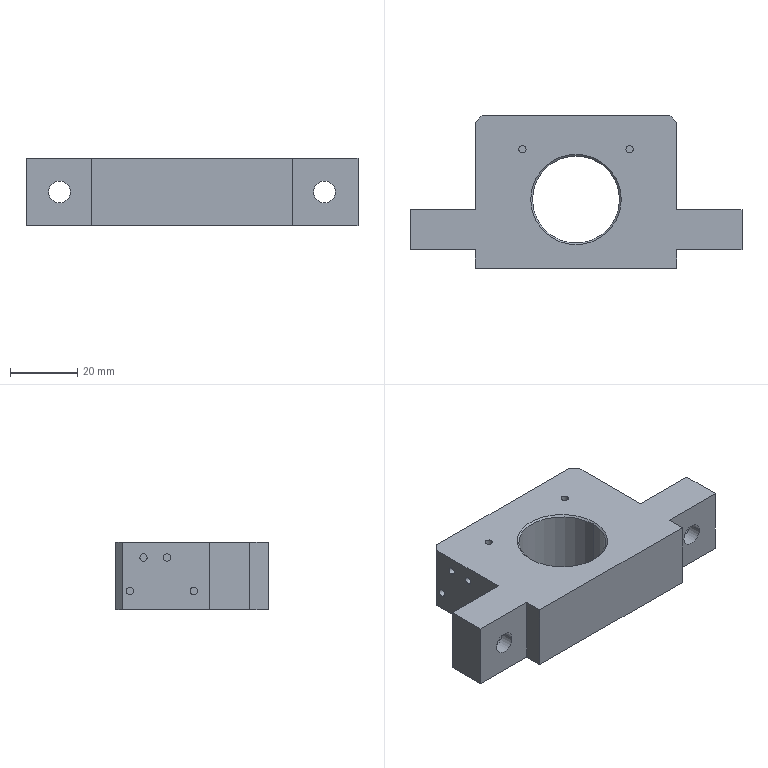Part | STEP file | SM140A-20-1140D-140A-600 Rear bearing seat | 1 solid | 48 faces | box 99 x 45.5 x 20 mm | volume 51169 mm3 | plane 24 | cylinder 22 | cone 2 | commonest cylinder face diameters 2.2 x12 6.5 x4 11 x4 26 x2